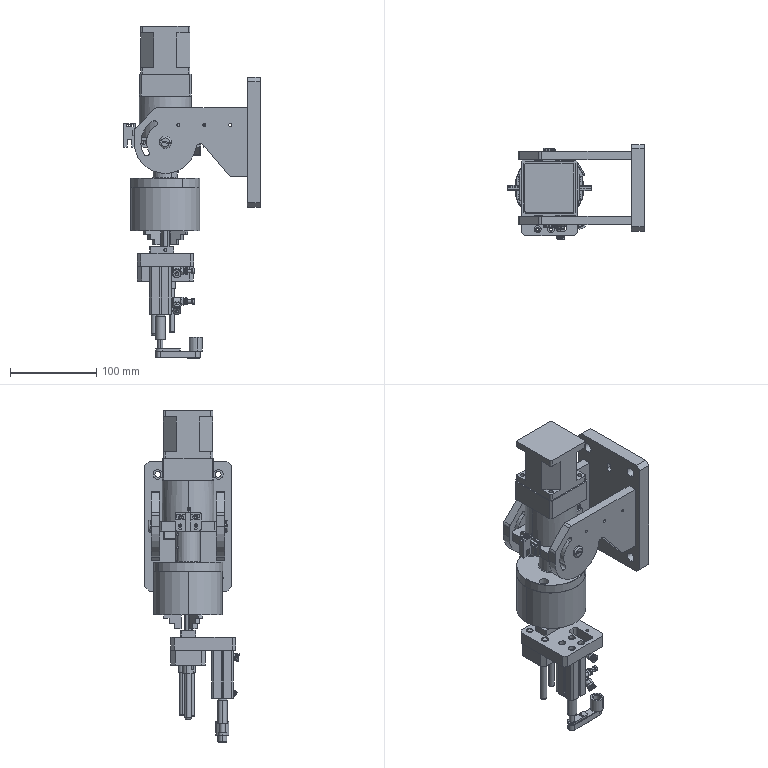Part | SolidWorks | 34 solids | 1429 faces | box 158.2 x 109.159 x 384 mm | volume 1286706 mm3 | plane 596 | cylinder 589 | cone 210 | spline 18 | torus 10 | sphere 6 | commonest cylinder face diameters 8 x54 3.3 x50 10 x37 5 x34 4 x28 6.5 x28